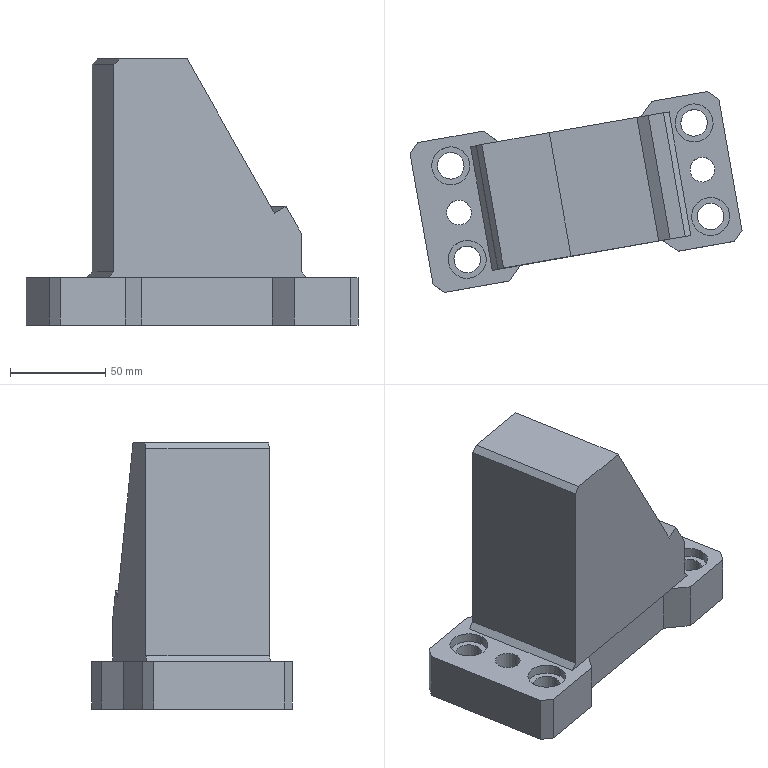Part | NX | features solid 2 | 1 solid | 46 faces | box 174.649 x 105.7 x 140 mm | volume 820537 mm3 | plane 36 | cylinder 10 | commonest cylinder face diameters 14 x4 20 x4 13 x2
STEP:
#1=CARTESIAN_POINT('',(-1147.121,323.745,25.));
#2=VERTEX_POINT('',#1);
#3=CARTESIAN_POINT('',(-1159.277,392.681,25.));
#4=VERTEX_POINT('',#3);
#5=CARTESIAN_POINT('',(-1153.199,358.213,25.));
#6=DIRECTION('',(-0.1736,0.9848,0.));
#7=VECTOR('',#6,1000.);
#8=LINE('',#5,#7);
#9=EDGE_CURVE('',#2,#4,#8,.T.);
#10=ORIENTED_EDGE('',*,*,#9,.F.);
#11=CARTESIAN_POINT('',(-1141.329,319.689,25.));
#12=VERTEX_POINT('',#11);
#13=CARTESIAN_POINT('',(-1119.608,304.48,25.));
#14=DIRECTION('',(-0.8192,0.5736,0.));
#15=VECTOR('',#14,1000.);
#16=LINE('',#13,#15);
#17=EDGE_CURVE('',#2,#12,#16,.F.);
#18=ORIENTED_EDGE('',*,*,#17,.T.);
#19=CARTESIAN_POINT('',(-1106.861,325.767,25.));
#20=VERTEX_POINT('',#19);
#21=CARTESIAN_POINT('',(-1065.007,333.147,25.));
#22=DIRECTION('',(-0.9848,-0.1736,0.));
#23=VECTOR('',#22,1000.);
#24=LINE('',#21,#23);
#25=EDGE_CURVE('',#20,#12,#24,.T.);
#26=ORIENTED_EDGE('',*,*,#25,.F.);
#27=CARTESIAN_POINT('',(-1101.183,333.876,25.));
#28=VERTEX_POINT('',#27);
#29=CARTESIAN_POINT('',(-1098.749,337.351,25.));
#30=DIRECTION('',(-0.5736,-0.8192,0.));
#31=VECTOR('',#30,1000.);
#32=LINE('',#29,#31);
#33=EDGE_CURVE('',#28,#20,#32,.T.);
#34=ORIENTED_EDGE('',*,*,#33,.F.);
#35=CARTESIAN_POINT('',(-1115.955,331.271,25.));
#36=VERTEX_POINT('',#35);
#37=CARTESIAN_POINT('',(-1113.,331.792,25.));
#38=DIRECTION('',(0.9848,0.1736,0.));
#39=VECTOR('',#38,1000.);
#40=LINE('',#37,#39);
#41=EDGE_CURVE('',#36,#28,#40,.T.);
#42=ORIENTED_EDGE('',*,*,#41,.F.);
#43=CARTESIAN_POINT('',(-1127.416,396.269,25.));
#44=VERTEX_POINT('',#43);
#45=CARTESIAN_POINT('',(-1127.416,396.269,25.));
#46=DIRECTION('',(-0.1736,0.9848,0.));
#47=VECTOR('',#46,1000.);
#48=LINE('',#45,#47);
#49=EDGE_CURVE('',#36,#44,#48,.T.);
#50=ORIENTED_EDGE('',*,*,#49,.T.);
#51=CARTESIAN_POINT('',(-1112.644,398.873,25.));
#52=VERTEX_POINT('',#51);
#53=CARTESIAN_POINT('',(-1124.461,396.79,25.));
#54=DIRECTION('',(0.9848,0.1736,0.));
#55=VECTOR('',#54,1000.);
#56=LINE('',#53,#55);
#57=EDGE_CURVE('',#44,#52,#56,.T.);
#58=ORIENTED_EDGE('',*,*,#57,.T.);
#59=CARTESIAN_POINT('',(-1120.753,404.551,25.));
#60=VERTEX_POINT('',#59);
#61=CARTESIAN_POINT('',(-1120.753,404.551,25.));
#62=DIRECTION('',(0.8192,-0.5736,0.));
#63=VECTOR('',#62,1000.);
#64=LINE('',#61,#63);
#65=EDGE_CURVE('',#60,#52,#64,.T.);
#66=ORIENTED_EDGE('',*,*,#65,.F.);
#67=CARTESIAN_POINT('',(-1155.221,398.474,25.));
#68=VERTEX_POINT('',#67);
#69=CARTESIAN_POINT('',(-1078.898,411.931,25.));
#70=DIRECTION('',(0.9848,0.1736,0.));
#71=VECTOR('',#70,1000.);
#72=LINE('',#69,#71);
#73=EDGE_CURVE('',#68,#60,#72,.T.);
#74=ORIENTED_EDGE('',*,*,#73,.F.);
#75=CARTESIAN_POINT('',(-1140.012,420.195,25.));
#76=DIRECTION('',(0.5736,0.8192,0.));
#77=VECTOR('',#76,1000.);
#78=LINE('',#75,#77);
#79=EDGE_CURVE('',#68,#4,#78,.F.);
#80=ORIENTED_EDGE('',*,*,#79,.T.);
#81=EDGE_LOOP('',(#10,#18,#26,#34,#42,#50,#58,#66,#74,#80));
#82=FACE_BOUND('',#81,.T.);
#83=CARTESIAN_POINT('',(-1127.996,388.043,25.));
#84=VERTEX_POINT('',#83);
#85=CARTESIAN_POINT('',(-1137.844,386.306,25.));
#86=DIRECTION('',(0.,0.,1.));
#87=DIRECTION('',(0.9848,0.1736,0.));
#88=AXIS2_PLACEMENT_3D('',#85,#86,#87);
#89=CIRCLE('',#88,10.);
#90=EDGE_CURVE('',#84,#84,#89,.T.);
#91=ORIENTED_EDGE('',*,*,#90,.F.);
#92=EDGE_LOOP('',(#91));
#93=FACE_BOUND('',#92,.T.);
#94=CARTESIAN_POINT('',(-1127.102,362.815,25.));
#95=VERTEX_POINT('',#94);
#96=CARTESIAN_POINT('',(-1133.503,361.686,25.));
#97=DIRECTION('',(0.,0.,1.));
#98=DIRECTION('',(0.9848,0.1736,0.));
#99=AXIS2_PLACEMENT_3D('',#96,#97,#98);
#100=CIRCLE('',#99,6.5);
#101=EDGE_CURVE('',#95,#95,#100,.T.);
#102=ORIENTED_EDGE('',*,*,#101,.F.);
#103=EDGE_LOOP('',(#102));
#104=FACE_BOUND('',#103,.T.);
#105=CARTESIAN_POINT('',(-1119.314,338.802,25.));
#106=VERTEX_POINT('',#105);
#107=CARTESIAN_POINT('',(-1129.162,337.066,25.));
#108=DIRECTION('',(0.,0.,1.));
#109=DIRECTION('',(0.9848,0.1736,0.));
#110=AXIS2_PLACEMENT_3D('',#107,#108,#109);
#111=CIRCLE('',#110,10.);
#112=EDGE_CURVE('',#106,#106,#111,.T.);
#113=ORIENTED_EDGE('',*,*,#112,.F.);
#114=EDGE_LOOP('',(#113));
#115=FACE_BOUND('',#114,.T.);
#116=CARTESIAN_POINT('',(-1071.952,372.539,25.));
#117=DIRECTION('',(0.,0.,1.));
#118=DIRECTION('',(0.9848,0.1736,0.));
#119=AXIS2_PLACEMENT_3D('',#116,#117,#118);
#120=PLANE('',#119);
#121=ADVANCED_FACE('',(#82,#93,#104,#115),#120,.T.);
#122=CARTESIAN_POINT('',(-996.784,421.333,25.));
#123=VERTEX_POINT('',#122);
#124=CARTESIAN_POINT('',(-984.628,352.397,25.));
#125=VERTEX_POINT('',#124);
#126=CARTESIAN_POINT('',(-990.706,386.865,25.));
#127=DIRECTION('',(0.1736,-0.9848,0.));
#128=VECTOR('',#127,1000.);
#129=LINE('',#126,#128);
#130=EDGE_CURVE('',#123,#125,#129,.T.);
#131=ORIENTED_EDGE('',*,*,#130,.F.);
#132=CARTESIAN_POINT('',(-1002.576,425.389,25.));
#133=VERTEX_POINT('',#132);
#134=CARTESIAN_POINT('',(-1024.297,440.598,25.));
#135=DIRECTION('',(0.8192,-0.5736,0.));
#136=VECTOR('',#135,1000.);
#137=LINE('',#134,#136);
#138=EDGE_CURVE('',#123,#133,#137,.F.);
#139=ORIENTED_EDGE('',*,*,#138,.T.);
#140=CARTESIAN_POINT('',(-1032.12,420.18,25.));
#141=VERTEX_POINT('',#140);
#142=CARTESIAN_POINT('',(-1078.898,411.931,25.));
#143=DIRECTION('',(0.9848,0.1736,0.));
#144=VECTOR('',#143,1000.);
#145=LINE('',#142,#144);
#146=EDGE_CURVE('',#141,#133,#145,.T.);
#147=ORIENTED_EDGE('',*,*,#146,.F.);
#148=CARTESIAN_POINT('',(-1037.798,412.071,25.));
#149=VERTEX_POINT('',#148);
#150=CARTESIAN_POINT('',(-1032.12,420.18,25.));
#151=DIRECTION('',(-0.5736,-0.8192,0.));
#152=VECTOR('',#151,1000.);
#153=LINE('',#150,#152);
#154=EDGE_CURVE('',#141,#149,#153,.T.);
#155=ORIENTED_EDGE('',*,*,#154,.T.);
#156=CARTESIAN_POINT('',(-1023.026,414.675,25.));
#157=VERTEX_POINT('',#156);
#158=CARTESIAN_POINT('',(-1124.461,396.79,25.));
#159=DIRECTION('',(0.9848,0.1736,0.));
#160=VECTOR('',#159,1000.);
#161=LINE('',#158,#160);
#162=EDGE_CURVE('',#149,#157,#161,.T.);
#163=ORIENTED_EDGE('',*,*,#162,.T.);
#164=CARTESIAN_POINT('',(-1011.565,349.678,25.));
#165=VERTEX_POINT('',#164);
#166=CARTESIAN_POINT('',(-1011.565,349.678,25.));
#167=DIRECTION('',(0.1736,-0.9848,0.));
#168=VECTOR('',#167,1000.);
#169=LINE('',#166,#168);
#170=EDGE_CURVE('',#157,#165,#169,.T.);
#171=ORIENTED_EDGE('',*,*,#170,.T.);
#172=CARTESIAN_POINT('',(-1026.337,347.073,25.));
#173=VERTEX_POINT('',#172);
#174=CARTESIAN_POINT('',(-1113.,331.792,25.));
#175=DIRECTION('',(0.9848,0.1736,0.));
#176=VECTOR('',#175,1000.);
#177=LINE('',#174,#176);
#178=EDGE_CURVE('',#173,#165,#177,.T.);
#179=ORIENTED_EDGE('',*,*,#178,.F.);
#180=CARTESIAN_POINT('',(-1018.228,341.395,25.));
#181=VERTEX_POINT('',#180);
#182=CARTESIAN_POINT('',(-1029.813,349.507,25.));
#183=DIRECTION('',(0.8192,-0.5736,0.));
#184=VECTOR('',#183,1000.);
#185=LINE('',#182,#184);
#186=EDGE_CURVE('',#173,#181,#185,.T.);
#187=ORIENTED_EDGE('',*,*,#186,.T.);
#188=CARTESIAN_POINT('',(-988.684,346.605,25.));
#189=VERTEX_POINT('',#188);
#190=CARTESIAN_POINT('',(-1065.007,333.147,25.));
#191=DIRECTION('',(-0.9848,-0.1736,0.));
#192=VECTOR('',#191,1000.);
#193=LINE('',#190,#192);
#194=EDGE_CURVE('',#189,#181,#193,.T.);
#195=ORIENTED_EDGE('',*,*,#194,.F.);
#196=CARTESIAN_POINT('',(-1003.893,324.884,25.));
#197=DIRECTION('',(-0.5736,-0.8192,0.));
#198=VECTOR('',#197,1000.);
#199=LINE('',#196,#198);
#200=EDGE_CURVE('',#189,#125,#199,.F.);
#201=ORIENTED_EDGE('',*,*,#200,.T.);
#202=EDGE_LOOP('',(#131,#139,#147,#155,#163,#171,#179,#187,#195,#201));
#203=FACE_BOUND('',#202,.T.);
#204=CARTESIAN_POINT('',(-999.971,410.617,25.));
#205=VERTEX_POINT('',#204);
#206=CARTESIAN_POINT('',(-1009.819,408.881,25.));
#207=DIRECTION('',(0.,0.,1.));
#208=DIRECTION('',(0.9848,0.1736,0.));
#209=AXIS2_PLACEMENT_3D('',#206,#207,#208);
#210=CIRCLE('',#209,10.);
#211=EDGE_CURVE('',#205,#205,#210,.T.);
#212=ORIENTED_EDGE('',*,*,#211,.F.);
#213=EDGE_LOOP('',(#212));
#214=FACE_BOUND('',#213,.T.);
#215=CARTESIAN_POINT('',(-999.077,385.389,25.));
#216=VERTEX_POINT('',#215);
#217=CARTESIAN_POINT('',(-1005.478,384.26,25.));
#218=DIRECTION('',(0.,0.,1.));
#219=DIRECTION('',(0.9848,0.1736,0.));
#220=AXIS2_PLACEMENT_3D('',#217,#218,#219);
#221=CIRCLE('',#220,6.5);
#222=EDGE_CURVE('',#216,#216,#221,.T.);
#223=ORIENTED_EDGE('',*,*,#222,.F.);
#224=EDGE_LOOP('',(#223));
#225=FACE_BOUND('',#224,.T.);
#226=CARTESIAN_POINT('',(-991.289,361.377,25.));
#227=VERTEX_POINT('',#226);
#228=CARTESIAN_POINT('',(-1001.137,359.64,25.));
#229=DIRECTION('',(0.,0.,1.));
#230=DIRECTION('',(0.9848,0.1736,0.));
#231=AXIS2_PLACEMENT_3D('',#228,#229,#230);
#232=CIRCLE('',#231,10.);
#233=EDGE_CURVE('',#227,#227,#232,.T.);
#234=ORIENTED_EDGE('',*,*,#233,.F.);
#235=EDGE_LOOP('',(#234));
#236=FACE_BOUND('',#235,.T.);
#237=CARTESIAN_POINT('',(-1071.952,372.539,25.));
#238=DIRECTION('',(0.,0.,1.));
#239=DIRECTION('',(0.9848,0.1736,0.));
#240=AXIS2_PLACEMENT_3D('',#237,#238,#239);
#241=PLANE('',#240);
#242=ADVANCED_FACE('',(#203,#214,#225,#236),#241,.T.);
#243=CARTESIAN_POINT('',(-1130.95,387.522,0.));
#244=VERTEX_POINT('',#243);
#245=CARTESIAN_POINT('',(-1137.844,386.306,0.));
#246=DIRECTION('',(0.,0.,1.));
#247=DIRECTION('',(0.9848,0.1736,0.));
#248=AXIS2_PLACEMENT_3D('',#245,#246,#247);
#249=CIRCLE('',#248,7.);
#250=EDGE_CURVE('',#244,#244,#249,.T.);
#251=ORIENTED_EDGE('',*,*,#250,.F.);
#252=EDGE_LOOP('',(#251));
#253=FACE_BOUND('',#252,.T.);
#254=CARTESIAN_POINT('',(-1144.738,385.091,20.));
#255=VERTEX_POINT('',#254);
#256=CARTESIAN_POINT('',(-1137.844,386.306,20.));
#257=DIRECTION('',(0.,0.,1.));
#258=DIRECTION('',(-0.9848,-0.1736,0.));
#259=AXIS2_PLACEMENT_3D('',#256,#257,#258);
#260=CIRCLE('',#259,7.);
#261=EDGE_CURVE('',#255,#255,#260,.T.);
#262=ORIENTED_EDGE('',*,*,#261,.T.);
#263=EDGE_LOOP('',(#262));
#264=FACE_BOUND('',#263,.T.);
#265=CARTESIAN_POINT('',(-1137.844,386.306,25.));
#266=DIRECTION('',(0.,0.,-1.));
#267=DIRECTION('',(-0.1736,0.9848,0.));
#268=AXIS2_PLACEMENT_3D('',#265,#266,#267);
#269=CYLINDRICAL_SURFACE('',#268,7.);
#270=ADVANCED_FACE('',(#253,#264),#269,.F.);
#271=CARTESIAN_POINT('',(-1122.268,338.282,0.));
#272=VERTEX_POINT('',#271);
#273=CARTESIAN_POINT('',(-1129.162,337.066,0.));
#274=DIRECTION('',(0.,0.,1.));
#275=DIRECTION('',(0.9848,0.1736,0.));
#276=AXIS2_PLACEMENT_3D('',#273,#274,#275);
#277=CIRCLE('',#276,7.);
#278=EDGE_CURVE('',#272,#272,#277,.T.);
#279=ORIENTED_EDGE('',*,*,#278,.F.);
#280=EDGE_LOOP('',(#279));
#281=FACE_BOUND('',#280,.T.);
#282=CARTESIAN_POINT('',(-1136.055,335.85,20.));
#283=VERTEX_POINT('',#282);
#284=CARTESIAN_POINT('',(-1129.162,337.066,20.));
#285=DIRECTION('',(0.,0.,1.));
#286=DIRECTION('',(-0.9848,-0.1736,0.));
#287=AXIS2_PLACEMENT_3D('',#284,#285,#286);
#288=CIRCLE('',#287,7.);
#289=EDGE_CURVE('',#283,#283,#288,.T.);
#290=ORIENTED_EDGE('',*,*,#289,.T.);
#291=EDGE_LOOP('',(#290));
#292=FACE_BOUND('',#291,.T.);
#293=CARTESIAN_POINT('',(-1129.162,337.066,25.));
#294=DIRECTION('',(0.,0.,-1.));
#295=DIRECTION('',(-0.1736,0.9848,0.));
#296=AXIS2_PLACEMENT_3D('',#293,#294,#295);
#297=CYLINDRICAL_SURFACE('',#296,7.);
#298=ADVANCED_FACE('',(#281,#292),#297,.F.);
#299=CARTESIAN_POINT('',(-994.243,360.856,0.));
#300=VERTEX_POINT('',#299);
#301=CARTESIAN_POINT('',(-1001.137,359.64,0.));
#302=DIRECTION('',(0.,0.,1.));
#303=DIRECTION('',(0.9848,0.1736,0.));
#304=AXIS2_PLACEMENT_3D('',#301,#302,#303);
#305=CIRCLE('',#304,7.);
#306=EDGE_CURVE('',#300,#300,#305,.T.);
#307=ORIENTED_EDGE('',*,*,#306,.F.);
#308=EDGE_LOOP('',(#307));
#309=FACE_BOUND('',#308,.T.);
#310=CARTESIAN_POINT('',(-1008.03,358.425,20.));
#311=VERTEX_POINT('',#310);
#312=CARTESIAN_POINT('',(-1001.137,359.64,20.));
#313=DIRECTION('',(0.,0.,1.));
#314=DIRECTION('',(-0.9848,-0.1736,0.));
#315=AXIS2_PLACEMENT_3D('',#312,#313,#314);
#316=CIRCLE('',#315,7.);
#317=EDGE_CURVE('',#311,#311,#316,.T.);
#318=ORIENTED_EDGE('',*,*,#317,.T.);
#319=EDGE_LOOP('',(#318));
#320=FACE_BOUND('',#319,.T.);
#321=CARTESIAN_POINT('',(-1001.137,359.64,25.));
#322=DIRECTION('',(0.,0.,-1.));
#323=DIRECTION('',(-0.1736,0.9848,0.));
#324=AXIS2_PLACEMENT_3D('',#321,#322,#323);
#325=CYLINDRICAL_SURFACE('',#324,7.);
#326=ADVANCED_FACE('',(#309,#320),#325,.F.);
#327=CARTESIAN_POINT('',(-1002.925,410.096,0.));
#328=VERTEX_POINT('',#327);
#329=CARTESIAN_POINT('',(-1009.819,408.881,0.));
#330=DIRECTION('',(0.,0.,1.));
#331=DIRECTION('',(0.9848,0.1736,0.));
#332=AXIS2_PLACEMENT_3D('',#329,#330,#331);
#333=CIRCLE('',#332,7.);
#334=EDGE_CURVE('',#328,#328,#333,.T.);
#335=ORIENTED_EDGE('',*,*,#334,.F.);
#336=EDGE_LOOP('',(#335));
#337=FACE_BOUND('',#336,.T.);
#338=CARTESIAN_POINT('',(-1016.713,407.665,20.));
#339=VERTEX_POINT('',#338);
#340=CARTESIAN_POINT('',(-1009.819,408.881,20.));
#341=DIRECTION('',(0.,0.,1.));
#342=DIRECTION('',(-0.9848,-0.1736,0.));
#343=AXIS2_PLACEMENT_3D('',#340,#341,#342);
#344=CIRCLE('',#343,7.);
#345=EDGE_CURVE('',#339,#339,#344,.T.);
#346=ORIENTED_EDGE('',*,*,#345,.T.);
#347=EDGE_LOOP('',(#346));
#348=FACE_BOUND('',#347,.T.);
#349=CARTESIAN_POINT('',(-1009.819,408.881,25.));
#350=DIRECTION('',(0.,0.,-1.));
#351=DIRECTION('',(-0.1736,0.9848,0.));
#352=AXIS2_PLACEMENT_3D('',#349,#350,#351);
#353=CYLINDRICAL_SURFACE('',#352,7.);
#354=ADVANCED_FACE('',(#337,#348),#353,.F.);
#355=CARTESIAN_POINT('',(-1127.102,362.815,0.));
#356=VERTEX_POINT('',#355);
#357=CARTESIAN_POINT('',(-1133.503,361.686,0.));
#358=DIRECTION('',(0.,0.,1.));
#359=DIRECTION('',(0.9848,0.1736,0.));
#360=AXIS2_PLACEMENT_3D('',#357,#358,#359);
#361=CIRCLE('',#360,6.5);
#362=EDGE_CURVE('',#356,#356,#361,.T.);
#363=ORIENTED_EDGE('',*,*,#362,.T.);
#364=EDGE_LOOP('',(#363));
#365=FACE_BOUND('',#364,.T.);
#366=ORIENTED_EDGE('',*,*,#306,.T.);
#367=EDGE_LOOP('',(#366));
#368=FACE_BOUND('',#367,.T.);
#369=ORIENTED_EDGE('',*,*,#334,.T.);
#370=EDGE_LOOP('',(#369));
#371=FACE_BOUND('',#370,.T.);
#372=CARTESIAN_POINT('',(-1002.576,425.389,0.));
#373=VERTEX_POINT('',#372);
#374=CARTESIAN_POINT('',(-1032.12,420.18,0.));
#375=VERTEX_POINT('',#374);
#376=CARTESIAN_POINT('',(-1078.898,411.931,0.));
#377=DIRECTION('',(-0.9848,-0.1736,0.));
#378=VECTOR('',#377,1000.);
#379=LINE('',#376,#378);
#380=EDGE_CURVE('',#373,#375,#379,.T.);
#381=ORIENTED_EDGE('',*,*,#380,.F.);
#382=CARTESIAN_POINT('',(-996.784,421.333,0.));
#383=VERTEX_POINT('',#382);
#384=CARTESIAN_POINT('',(-1024.297,440.598,0.));
#385=DIRECTION('',(-0.8192,0.5736,0.));
#386=VECTOR('',#385,1000.);
#387=LINE('',#384,#386);
#388=EDGE_CURVE('',#373,#383,#387,.F.);
#389=ORIENTED_EDGE('',*,*,#388,.T.);
#390=CARTESIAN_POINT('',(-984.628,352.397,0.));
#391=VERTEX_POINT('',#390);
#392=CARTESIAN_POINT('',(-990.706,386.865,0.));
#393=DIRECTION('',(-0.1736,0.9848,0.));
#394=VECTOR('',#393,1000.);
#395=LINE('',#392,#394);
#396=EDGE_CURVE('',#391,#383,#395,.T.);
#397=ORIENTED_EDGE('',*,*,#396,.F.);
#398=CARTESIAN_POINT('',(-988.684,346.605,0.));
#399=VERTEX_POINT('',#398);
#400=CARTESIAN_POINT('',(-1003.893,324.884,0.));
#401=DIRECTION('',(0.5736,0.8192,0.));
#402=VECTOR('',#401,1000.);
#403=LINE('',#400,#402);
#404=EDGE_CURVE('',#391,#399,#403,.F.);
#405=ORIENTED_EDGE('',*,*,#404,.T.);
#406=CARTESIAN_POINT('',(-1018.228,341.395,0.));
#407=VERTEX_POINT('',#406);
#408=CARTESIAN_POINT('',(-1065.007,333.147,0.));
#409=DIRECTION('',(0.9848,0.1736,0.));
#410=VECTOR('',#409,1000.);
#411=LINE('',#408,#410);
#412=EDGE_CURVE('',#407,#399,#411,.T.);
#413=ORIENTED_EDGE('',*,*,#412,.F.);
#414=CARTESIAN_POINT('',(-1029.813,349.507,0.));
#415=VERTEX_POINT('',#414);
#416=CARTESIAN_POINT('',(-1029.813,349.507,0.));
#417=DIRECTION('',(0.8192,-0.5736,0.));
#418=VECTOR('',#417,1000.);
#419=LINE('',#416,#418);
#420=EDGE_CURVE('',#415,#407,#419,.T.);
#421=ORIENTED_EDGE('',*,*,#420,.F.);
#422=CARTESIAN_POINT('',(-1098.749,337.351,0.));
#423=VERTEX_POINT('',#422);
#424=CARTESIAN_POINT('',(-1098.749,337.351,0.));
#425=DIRECTION('',(0.9848,0.1736,0.));
#426=VECTOR('',#425,1000.);
#427=LINE('',#424,#426);
#428=EDGE_CURVE('',#423,#415,#427,.T.);
#429=ORIENTED_EDGE('',*,*,#428,.F.);
#430=CARTESIAN_POINT('',(-1106.861,325.767,0.));
#431=VERTEX_POINT('',#430);
#432=CARTESIAN_POINT('',(-1098.749,337.351,0.));
#433=DIRECTION('',(-0.5736,-0.8192,0.));
#434=VECTOR('',#433,1000.);
#435=LINE('',#432,#434);
#436=EDGE_CURVE('',#423,#431,#435,.T.);
#437=ORIENTED_EDGE('',*,*,#436,.T.);
#438=CARTESIAN_POINT('',(-1141.329,319.689,0.));
#439=VERTEX_POINT('',#438);
#440=CARTESIAN_POINT('',(-1065.007,333.147,0.));
#441=DIRECTION('',(0.9848,0.1736,0.));
#442=VECTOR('',#441,1000.);
#443=LINE('',#440,#442);
#444=EDGE_CURVE('',#439,#431,#443,.T.);
#445=ORIENTED_EDGE('',*,*,#444,.F.);
#446=CARTESIAN_POINT('',(-1147.121,323.745,0.));
#447=VERTEX_POINT('',#446);
#448=CARTESIAN_POINT('',(-1119.608,304.48,0.));
#449=DIRECTION('',(0.8192,-0.5736,0.));
#450=VECTOR('',#449,1000.);
#451=LINE('',#448,#450);
#452=EDGE_CURVE('',#439,#447,#451,.F.);
#453=ORIENTED_EDGE('',*,*,#452,.T.);
#454=CARTESIAN_POINT('',(-1159.277,392.681,0.));
#455=VERTEX_POINT('',#454);
#456=CARTESIAN_POINT('',(-1153.199,358.213,0.));
#457=DIRECTION('',(0.1736,-0.9848,0.));
#458=VECTOR('',#457,1000.);
#459=LINE('',#456,#458);
#460=EDGE_CURVE('',#455,#447,#459,.T.);
#461=ORIENTED_EDGE('',*,*,#460,.F.);
#462=CARTESIAN_POINT('',(-1155.221,398.474,0.));
#463=VERTEX_POINT('',#462);
#464=CARTESIAN_POINT('',(-1140.012,420.195,0.));
#465=DIRECTION('',(-0.5736,-0.8192,0.));
#466=VECTOR('',#465,1000.);
#467=LINE('',#464,#466);
#468=EDGE_CURVE('',#455,#463,#467,.F.);
#469=ORIENTED_EDGE('',*,*,#468,.T.);
#470=CARTESIAN_POINT('',(-1120.753,404.551,0.));
#471=VERTEX_POINT('',#470);
#472=CARTESIAN_POINT('',(-1078.898,411.931,0.));
#473=DIRECTION('',(-0.9848,-0.1736,0.));
#474=VECTOR('',#473,1000.);
#475=LINE('',#472,#474);
#476=EDGE_CURVE('',#471,#463,#475,.T.);
#477=ORIENTED_EDGE('',*,*,#476,.F.);
#478=CARTESIAN_POINT('',(-1109.168,396.44,0.));
#479=VERTEX_POINT('',#478);
#480=CARTESIAN_POINT('',(-1120.753,404.551,0.));
#481=DIRECTION('',(0.8192,-0.5736,0.));
#482=VECTOR('',#481,1000.);
#483=LINE('',#480,#482);
#484=EDGE_CURVE('',#471,#479,#483,.T.);
#485=ORIENTED_EDGE('',*,*,#484,.T.);
#486=CARTESIAN_POINT('',(-1040.232,408.595,0.));
#487=VERTEX_POINT('',#486);
#488=CARTESIAN_POINT('',(-1109.168,396.44,0.));
#489=DIRECTION('',(0.9848,0.1736,0.));
#490=VECTOR('',#489,1000.);
#491=LINE('',#488,#490);
#492=EDGE_CURVE('',#479,#487,#491,.T.);
#493=ORIENTED_EDGE('',*,*,#492,.T.);
#494=CARTESIAN_POINT('',(-1032.12,420.18,0.));
#495=DIRECTION('',(-0.5736,-0.8192,0.));
#496=VECTOR('',#495,1000.);
#497=LINE('',#494,#496);
#498=EDGE_CURVE('',#375,#487,#497,.T.);
#499=ORIENTED_EDGE('',*,*,#498,.F.);
#500=EDGE_LOOP('',(#381,#389,#397,#405,#413,#421,#429,#437,#445,#453,#461,#469,#477,#485,#493,#499));
#501=FACE_BOUND('',#500,.T.);
#502=CARTESIAN_POINT('',(-999.077,385.389,0.));
#503=VERTEX_POINT('',#502);
#504=CARTESIAN_POINT('',(-1005.478,384.26,0.));
#505=DIRECTION('',(0.,0.,1.));
#506=DIRECTION('',(0.9848,0.1736,0.));
#507=AXIS2_PLACEMENT_3D('',#504,#505,#506);
#508=CIRCLE('',#507,6.5);
#509=EDGE_CURVE('',#503,#503,#508,.T.);
#510=ORIENTED_EDGE('',*,*,#509,.T.);
#511=EDGE_LOOP('',(#510));
#512=FACE_BOUND('',#511,.T.);
#513=ORIENTED_EDGE('',*,*,#250,.T.);
#514=EDGE_LOOP('',(#513));
#515=FACE_BOUND('',#514,.T.);
#516=ORIENTED_EDGE('',*,*,#278,.T.);
#517=EDGE_LOOP('',(#516));
#518=FACE_BOUND('',#517,.T.);
#519=CARTESIAN_POINT('',(-1071.952,372.539,0.));
#520=DIRECTION('',(0.,0.,-1.));
#521=DIRECTION('',(-0.9848,-0.1736,0.));
#522=AXIS2_PLACEMENT_3D('',#519,#520,#521);
#523=PLANE('',#522);
#524=ADVANCED_FACE('',(#365,#368,#371,#501,#512,#515,#518),#523,.T.);
#525=ORIENTED_EDGE('',*,*,#25,.T.);
#526=CARTESIAN_POINT('',(-1141.329,319.689,0.));
#527=DIRECTION('',(0.,0.,-1.));
#528=VECTOR('',#527,1000.);
#529=LINE('',#526,#528);
#530=EDGE_CURVE('',#12,#439,#529,.T.);
#531=ORIENTED_EDGE('',*,*,#530,.T.);
#532=ORIENTED_EDGE('',*,*,#444,.T.);
#533=CARTESIAN_POINT('',(-1106.861,325.767,25.));
#534=DIRECTION('',(0.,0.,-1.));
#535=VECTOR('',#534,1000.);
#536=LINE('',#533,#535);
#537=EDGE_CURVE('',#20,#431,#536,.T.);
#538=ORIENTED_EDGE('',*,*,#537,.F.);
#539=EDGE_LOOP('',(#525,#531,#532,#538));
#540=FACE_BOUND('',#539,.T.);
#541=CARTESIAN_POINT('',(-1065.007,333.147,0.));
#542=DIRECTION('',(0.1736,-0.9848,0.));
#543=DIRECTION('',(0.,0.,-1.));
#544=AXIS2_PLACEMENT_3D('',#541,#542,#543);
#545=PLANE('',#544);
#546=ADVANCED_FACE('',(#540),#545,.T.);
#547=ORIENTED_EDGE('',*,*,#476,.T.);
#548=CARTESIAN_POINT('',(-1155.221,398.474,0.));
#549=DIRECTION('',(0.,0.,1.));
#550=VECTOR('',#549,1000.);
#551=LINE('',#548,#550);
#552=EDGE_CURVE('',#463,#68,#551,.T.);
#553=ORIENTED_EDGE('',*,*,#552,.T.);
#554=ORIENTED_EDGE('',*,*,#73,.T.);
#555=CARTESIAN_POINT('',(-1120.753,404.551,25.));
#556=DIRECTION('',(0.,0.,-1.));
#557=VECTOR('',#556,1000.);
#558=LINE('',#555,#557);
#559=EDGE_CURVE('',#60,#471,#558,.T.);
#560=ORIENTED_EDGE('',*,*,#559,.T.);
#561=EDGE_LOOP('',(#547,#553,#554,#560));
#562=FACE_BOUND('',#561,.T.);
#563=CARTESIAN_POINT('',(-1078.898,411.931,0.));
#564=DIRECTION('',(-0.1736,0.9848,0.));
#565=DIRECTION('',(0.,0.,1.));
#566=AXIS2_PLACEMENT_3D('',#563,#564,#565);
#567=PLANE('',#566);
#568=ADVANCED_FACE('',(#562),#567,.T.);
#569=ORIENTED_EDGE('',*,*,#412,.T.);
#570=CARTESIAN_POINT('',(-988.684,346.605,0.));
#571=DIRECTION('',(0.,0.,1.));
#572=VECTOR('',#571,1000.);
#573=LINE('',#570,#572);
#574=EDGE_CURVE('',#399,#189,#573,.T.);
#575=ORIENTED_EDGE('',*,*,#574,.T.);
#576=ORIENTED_EDGE('',*,*,#194,.T.);
#577=CARTESIAN_POINT('',(-1018.228,341.395,25.));
#578=DIRECTION('',(0.,0.,-1.));
#579=VECTOR('',#578,1000.);
#580=LINE('',#577,#579);
#581=EDGE_CURVE('',#181,#407,#580,.T.);
#582=ORIENTED_EDGE('',*,*,#581,.T.);
#583=EDGE_LOOP('',(#569,#575,#576,#582));
#584=FACE_BOUND('',#583,.T.);
#585=CARTESIAN_POINT('',(-1065.007,333.147,0.));
#586=DIRECTION('',(0.1736,-0.9848,0.));
#587=DIRECTION('',(0.,0.,-1.));
#588=AXIS2_PLACEMENT_3D('',#585,#586,#587);
#589=PLANE('',#588);
#590=ADVANCED_FACE('',(#584),#589,.T.);
#591=ORIENTED_EDGE('',*,*,#460,.T.);
#592=CARTESIAN_POINT('',(-1147.121,323.745,0.));
#593=DIRECTION('',(0.,0.,1.));
#594=VECTOR('',#593,1000.);
#595=LINE('',#592,#594);
#596=EDGE_CURVE('',#447,#2,#595,.T.);
#597=ORIENTED_EDGE('',*,*,#596,.T.);
#598=ORIENTED_EDGE('',*,*,#9,.T.);
#599=CARTESIAN_POINT('',(-1159.277,392.681,0.));
#600=DIRECTION('',(0.,0.,-1.));
#601=VECTOR('',#600,1000.);
#602=LINE('',#599,#601);
#603=EDGE_CURVE('',#4,#455,#602,.T.);
#604=ORIENTED_EDGE('',*,*,#603,.T.);
#605=EDGE_LOOP('',(#591,#597,#598,#604));
#606=FACE_BOUND('',#605,.T.);
#607=CARTESIAN_POINT('',(-1153.199,358.213,0.));
#608=DIRECTION('',(-0.9848,-0.1736,0.));
#609=DIRECTION('',(0.,0.,1.));
#610=AXIS2_PLACEMENT_3D('',#607,#608,#609);
#611=PLANE('',#610);
#612=ADVANCED_FACE('',(#606),#611,.T.);
#613=ORIENTED_EDGE('',*,*,#146,.T.);
#614=CARTESIAN_POINT('',(-1002.576,425.389,0.));
#615=DIRECTION('',(0.,0.,-1.));
#616=VECTOR('',#615,1000.);
#617=LINE('',#614,#616);
#618=EDGE_CURVE('',#133,#373,#617,.T.);
#619=ORIENTED_EDGE('',*,*,#618,.T.);
#620=ORIENTED_EDGE('',*,*,#380,.T.);
#621=CARTESIAN_POINT('',(-1032.12,420.18,25.));
#622=DIRECTION('',(0.,0.,-1.));
#623=VECTOR('',#622,1000.);
#624=LINE('',#621,#623);
#625=EDGE_CURVE('',#141,#375,#624,.T.);
#626=ORIENTED_EDGE('',*,*,#625,.F.);
#627=EDGE_LOOP('',(#613,#619,#620,#626));
#628=FACE_BOUND('',#627,.T.);
#629=CARTESIAN_POINT('',(-1078.898,411.931,0.));
#630=DIRECTION('',(-0.1736,0.9848,0.));
#631=DIRECTION('',(0.,0.,1.));
#632=AXIS2_PLACEMENT_3D('',#629,#630,#631);
#633=PLANE('',#632);
#634=ADVANCED_FACE('',(#628),#633,.T.);
#635=ORIENTED_EDGE('',*,*,#396,.T.);
#636=CARTESIAN_POINT('',(-996.784,421.333,0.));
#637=DIRECTION('',(0.,0.,1.));
#638=VECTOR('',#637,1000.);
#639=LINE('',#636,#638);
#640=EDGE_CURVE('',#383,#123,#639,.T.);
#641=ORIENTED_EDGE('',*,*,#640,.T.);
#642=ORIENTED_EDGE('',*,*,#130,.T.);
#643=CARTESIAN_POINT('',(-984.628,352.397,0.));
#644=DIRECTION('',(0.,0.,-1.));
#645=VECTOR('',#644,1000.);
#646=LINE('',#643,#645);
#647=EDGE_CURVE('',#125,#391,#646,.T.);
#648=ORIENTED_EDGE('',*,*,#647,.T.);
#649=EDGE_LOOP('',(#635,#641,#642,#648));
#650=FACE_BOUND('',#649,.T.);
#651=CARTESIAN_POINT('',(-990.706,386.865,0.));
#652=DIRECTION('',(0.9848,0.1736,0.));
#653=DIRECTION('',(0.,0.,-1.));
#654=AXIS2_PLACEMENT_3D('',#651,#652,#653);
#655=PLANE('',#654);
#656=ADVANCED_FACE('',(#650),#655,.T.);
#657=ORIENTED_EDGE('',*,*,#498,.T.);
#658=CARTESIAN_POINT('',(-1040.232,408.595,25.));
#659=VERTEX_POINT('',#658);
#660=CARTESIAN_POINT('',(-1040.232,408.595,25.));
#661=DIRECTION('',(0.,0.,-1.));
#662=VECTOR('',#661,1000.);
#663=LINE('',#660,#662);
#664=EDGE_CURVE('',#659,#487,#663,.T.);
#665=ORIENTED_EDGE('',*,*,#664,.F.);
#666=CARTESIAN_POINT('',(-1032.12,420.18,25.));
#667=DIRECTION('',(-0.5736,-0.8192,0.));
#668=VECTOR('',#667,1000.);
#669=LINE('',#666,#668);
#670=EDGE_CURVE('',#149,#659,#669,.T.);
#671=ORIENTED_EDGE('',*,*,#670,.F.);
#672=ORIENTED_EDGE('',*,*,#154,.F.);
#673=ORIENTED_EDGE('',*,*,#625,.T.);
#674=EDGE_LOOP('',(#657,#665,#671,#672,#673));
#675=FACE_BOUND('',#674,.T.);
#676=CARTESIAN_POINT('',(-1032.12,420.18,25.));
#677=DIRECTION('',(0.8192,-0.5736,0.));
#678=DIRECTION('',(0.5736,0.8192,0.));
#679=AXIS2_PLACEMENT_3D('',#676,#677,#678);
#680=PLANE('',#679);
#681=ADVANCED_FACE('',(#675),#680,.F.);
#682=ORIENTED_EDGE('',*,*,#492,.F.);
#683=CARTESIAN_POINT('',(-1109.168,396.44,25.));
#684=VERTEX_POINT('',#683);
#685=CARTESIAN_POINT('',(-1109.168,396.44,25.));
#686=DIRECTION('',(0.,0.,-1.));
#687=VECTOR('',#686,1000.);
#688=LINE('',#685,#687);
#689=EDGE_CURVE('',#684,#479,#688,.T.);
#690=ORIENTED_EDGE('',*,*,#689,.F.);
#691=CARTESIAN_POINT('',(-1109.168,396.44,25.));
#692=DIRECTION('',(0.9848,0.1736,0.));
#693=VECTOR('',#692,1000.);
#694=LINE('',#691,#693);
#695=EDGE_CURVE('',#684,#659,#694,.T.);
#696=ORIENTED_EDGE('',*,*,#695,.T.);
#697=ORIENTED_EDGE('',*,*,#664,.T.);
#698=EDGE_LOOP('',(#682,#690,#696,#697));
#699=FACE_BOUND('',#698,.T.);
#700=CARTESIAN_POINT('',(-1109.168,396.44,25.));
#701=DIRECTION('',(-0.1736,0.9848,0.));
#702=DIRECTION('',(-0.9848,-0.1736,0.));
#703=AXIS2_PLACEMENT_3D('',#700,#701,#702);
#704=PLANE('',#703);
#705=ADVANCED_FACE('',(#699),#704,.T.);
#706=ORIENTED_EDGE('',*,*,#484,.F.);
#707=ORIENTED_EDGE('',*,*,#559,.F.);
#708=ORIENTED_EDGE('',*,*,#65,.T.);
#709=CARTESIAN_POINT('',(-1120.753,404.551,25.));
#710=DIRECTION('',(0.8192,-0.5736,0.));
#711=VECTOR('',#710,1000.);
#712=LINE('',#709,#711);
#713=EDGE_CURVE('',#52,#684,#712,.T.);
#714=ORIENTED_EDGE('',*,*,#713,.T.);
#715=ORIENTED_EDGE('',*,*,#689,.T.);
#716=EDGE_LOOP('',(#706,#707,#708,#714,#715));
#717=FACE_BOUND('',#716,.T.);
#718=CARTESIAN_POINT('',(-1120.753,404.551,25.));
#719=DIRECTION('',(0.5736,0.8192,0.));
#720=DIRECTION('',(-0.8192,0.5736,0.));
#721=AXIS2_PLACEMENT_3D('',#718,#719,#720);
#722=PLANE('',#721);
#723=ADVANCED_FACE('',(#717),#722,.T.);
#724=ORIENTED_EDGE('',*,*,#420,.T.);
#725=ORIENTED_EDGE('',*,*,#581,.F.);
#726=ORIENTED_EDGE('',*,*,#186,.F.);
#727=CARTESIAN_POINT('',(-1029.813,349.507,25.));
#728=VERTEX_POINT('',#727);
#729=CARTESIAN_POINT('',(-1029.813,349.507,25.));
#730=DIRECTION('',(0.8192,-0.5736,0.));
#731=VECTOR('',#730,1000.);
#732=LINE('',#729,#731);
#733=EDGE_CURVE('',#728,#173,#732,.T.);
#734=ORIENTED_EDGE('',*,*,#733,.F.);
#735=CARTESIAN_POINT('',(-1029.813,349.507,25.));
#736=DIRECTION('',(0.,0.,-1.));
#737=VECTOR('',#736,1000.);
#738=LINE('',#735,#737);
#739=EDGE_CURVE('',#728,#415,#738,.T.);
#740=ORIENTED_EDGE('',*,*,#739,.T.);
#741=EDGE_LOOP('',(#724,#725,#726,#734,#740));
#742=FACE_BOUND('',#741,.T.);
#743=CARTESIAN_POINT('',(-1029.813,349.507,25.));
#744=DIRECTION('',(0.5736,0.8192,0.));
#745=DIRECTION('',(-0.8192,0.5736,0.));
#746=AXIS2_PLACEMENT_3D('',#743,#744,#745);
#747=PLANE('',#746);
#748=ADVANCED_FACE('',(#742),#747,.F.);
#749=ORIENTED_EDGE('',*,*,#436,.F.);
#750=CARTESIAN_POINT('',(-1098.749,337.351,25.));
#751=VERTEX_POINT('',#750);
#752=CARTESIAN_POINT('',(-1098.749,337.351,25.));
#753=DIRECTION('',(0.,0.,-1.));
#754=VECTOR('',#753,1000.);
#755=LINE('',#752,#754);
#756=EDGE_CURVE('',#751,#423,#755,.T.);
#757=ORIENTED_EDGE('',*,*,#756,.F.);
#758=CARTESIAN_POINT('',(-1098.749,337.351,25.));
#759=DIRECTION('',(-0.5736,-0.8192,0.));
#760=VECTOR('',#759,1000.);
#761=LINE('',#758,#760);
#762=EDGE_CURVE('',#751,#28,#761,.T.);
#763=ORIENTED_EDGE('',*,*,#762,.T.);
#764=ORIENTED_EDGE('',*,*,#33,.T.);
#765=ORIENTED_EDGE('',*,*,#537,.T.);
#766=EDGE_LOOP('',(#749,#757,#763,#764,#765));
#767=FACE_BOUND('',#766,.T.);
#768=CARTESIAN_POINT('',(-1098.749,337.351,25.));
#769=DIRECTION('',(0.8192,-0.5736,0.));
#770=DIRECTION('',(0.5736,0.8192,0.));
#771=AXIS2_PLACEMENT_3D('',#768,#769,#770);
#772=PLANE('',#771);
#773=ADVANCED_FACE('',(#767),#772,.T.);
#774=ORIENTED_EDGE('',*,*,#428,.T.);
#775=ORIENTED_EDGE('',*,*,#739,.F.);
#776=CARTESIAN_POINT('',(-1098.749,337.351,25.));
#777=DIRECTION('',(0.9848,0.1736,0.));
#778=VECTOR('',#777,1000.);
#779=LINE('',#776,#778);
#780=EDGE_CURVE('',#751,#728,#779,.T.);
#781=ORIENTED_EDGE('',*,*,#780,.F.);
#782=ORIENTED_EDGE('',*,*,#756,.T.);
#783=EDGE_LOOP('',(#774,#775,#781,#782));
#784=FACE_BOUND('',#783,.T.);
#785=CARTESIAN_POINT('',(-1098.749,337.351,25.));
#786=DIRECTION('',(-0.1736,0.9848,0.));
#787=DIRECTION('',(-0.9848,-0.1736,0.));
#788=AXIS2_PLACEMENT_3D('',#785,#786,#787);
#789=PLANE('',#788);
#790=ADVANCED_FACE('',(#784),#789,.F.);
#791=ORIENTED_EDGE('',*,*,#222,.T.);
#792=EDGE_LOOP('',(#791));
#793=FACE_BOUND('',#792,.T.);
#794=ORIENTED_EDGE('',*,*,#509,.F.);
#795=EDGE_LOOP('',(#794));
#796=FACE_BOUND('',#795,.T.);
#797=CARTESIAN_POINT('',(-1005.478,384.26,25.));
#798=DIRECTION('',(0.,0.,-1.));
#799=DIRECTION('',(-0.1736,0.9848,0.));
#800=AXIS2_PLACEMENT_3D('',#797,#798,#799);
#801=CYLINDRICAL_SURFACE('',#800,6.5);
#802=ADVANCED_FACE('',(#793,#796),#801,.F.);
#803=ORIENTED_EDGE('',*,*,#101,.T.);
#804=EDGE_LOOP('',(#803));
#805=FACE_BOUND('',#804,.T.);
#806=ORIENTED_EDGE('',*,*,#362,.F.);
#807=EDGE_LOOP('',(#806));
#808=FACE_BOUND('',#807,.T.);
#809=CARTESIAN_POINT('',(-1133.503,361.686,25.));
#810=DIRECTION('',(0.,0.,-1.));
#811=DIRECTION('',(-0.1736,0.9848,0.));
#812=AXIS2_PLACEMENT_3D('',#809,#810,#811);
#813=CYLINDRICAL_SURFACE('',#812,6.5);
#814=ADVANCED_FACE('',(#805,#808),#813,.F.);
#815=ORIENTED_EDGE('',*,*,#211,.T.);
#816=EDGE_LOOP('',(#815));
#817=FACE_BOUND('',#816,.T.);
#818=CARTESIAN_POINT('',(-999.971,410.617,20.));
#819=VERTEX_POINT('',#818);
#820=CARTESIAN_POINT('',(-1009.819,408.881,20.));
#821=DIRECTION('',(0.,0.,1.));
#822=DIRECTION('',(0.9848,0.1736,0.));
#823=AXIS2_PLACEMENT_3D('',#820,#821,#822);
#824=CIRCLE('',#823,10.);
#825=EDGE_CURVE('',#819,#819,#824,.T.);
#826=ORIENTED_EDGE('',*,*,#825,.F.);
#827=EDGE_LOOP('',(#826));
#828=FACE_BOUND('',#827,.T.);
#829=CARTESIAN_POINT('',(-1009.819,408.881,25.));
#830=DIRECTION('',(0.,0.,-1.));
#831=DIRECTION('',(-0.1736,0.9848,0.));
#832=AXIS2_PLACEMENT_3D('',#829,#830,#831);
#833=CYLINDRICAL_SURFACE('',#832,10.);
#834=ADVANCED_FACE('',(#817,#828),#833,.F.);
#835=ORIENTED_EDGE('',*,*,#345,.F.);
#836=EDGE_LOOP('',(#835));
#837=FACE_BOUND('',#836,.T.);
#838=ORIENTED_EDGE('',*,*,#825,.T.);
#839=EDGE_LOOP('',(#838));
#840=FACE_BOUND('',#839,.T.);
#841=CARTESIAN_POINT('',(-1009.819,408.881,20.));
#842=DIRECTION('',(0.,0.,1.));
#843=DIRECTION('',(-0.9848,-0.1736,0.));
#844=AXIS2_PLACEMENT_3D('',#841,#842,#843);
#845=PLANE('',#844);
#846=ADVANCED_FACE('',(#837,#840),#845,.T.);
#847=ORIENTED_EDGE('',*,*,#233,.T.);
#848=EDGE_LOOP('',(#847));
#849=FACE_BOUND('',#848,.T.);
#850=CARTESIAN_POINT('',(-991.289,361.377,20.));
#851=VERTEX_POINT('',#850);
#852=CARTESIAN_POINT('',(-1001.137,359.64,20.));
#853=DIRECTION('',(0.,0.,1.));
#854=DIRECTION('',(0.9848,0.1736,0.));
#855=AXIS2_PLACEMENT_3D('',#852,#853,#854);
#856=CIRCLE('',#855,10.);
#857=EDGE_CURVE('',#851,#851,#856,.T.);
#858=ORIENTED_EDGE('',*,*,#857,.F.);
#859=EDGE_LOOP('',(#858));
#860=FACE_BOUND('',#859,.T.);
#861=CARTESIAN_POINT('',(-1001.137,359.64,25.));
#862=DIRECTION('',(0.,0.,-1.));
#863=DIRECTION('',(-0.1736,0.9848,0.));
#864=AXIS2_PLACEMENT_3D('',#861,#862,#863);
#865=CYLINDRICAL_SURFACE('',#864,10.);
#866=ADVANCED_FACE('',(#849,#860),#865,.F.);
#867=ORIENTED_EDGE('',*,*,#317,.F.);
#868=EDGE_LOOP('',(#867));
#869=FACE_BOUND('',#868,.T.);
#870=ORIENTED_EDGE('',*,*,#857,.T.);
#871=EDGE_LOOP('',(#870));
#872=FACE_BOUND('',#871,.T.);
#873=CARTESIAN_POINT('',(-1001.137,359.64,20.));
#874=DIRECTION('',(0.,0.,1.));
#875=DIRECTION('',(-0.9848,-0.1736,0.));
#876=AXIS2_PLACEMENT_3D('',#873,#874,#875);
#877=PLANE('',#876);
#878=ADVANCED_FACE('',(#869,#872),#877,.T.);
#879=ORIENTED_EDGE('',*,*,#112,.T.);
#880=EDGE_LOOP('',(#879));
#881=FACE_BOUND('',#880,.T.);
#882=CARTESIAN_POINT('',(-1119.314,338.802,20.));
#883=VERTEX_POINT('',#882);
#884=CARTESIAN_POINT('',(-1129.162,337.066,20.));
#885=DIRECTION('',(0.,0.,1.));
#886=DIRECTION('',(0.9848,0.1736,0.));
#887=AXIS2_PLACEMENT_3D('',#884,#885,#886);
#888=CIRCLE('',#887,10.);
#889=EDGE_CURVE('',#883,#883,#888,.T.);
#890=ORIENTED_EDGE('',*,*,#889,.F.);
#891=EDGE_LOOP('',(#890));
#892=FACE_BOUND('',#891,.T.);
#893=CARTESIAN_POINT('',(-1129.162,337.066,25.));
#894=DIRECTION('',(0.,0.,-1.));
#895=DIRECTION('',(-0.1736,0.9848,0.));
#896=AXIS2_PLACEMENT_3D('',#893,#894,#895);
#897=CYLINDRICAL_SURFACE('',#896,10.);
#898=ADVANCED_FACE('',(#881,#892),#897,.F.);
#899=ORIENTED_EDGE('',*,*,#289,.F.);
#900=EDGE_LOOP('',(#899));
#901=FACE_BOUND('',#900,.T.);
#902=ORIENTED_EDGE('',*,*,#889,.T.);
#903=EDGE_LOOP('',(#902));
#904=FACE_BOUND('',#903,.T.);
#905=CARTESIAN_POINT('',(-1129.162,337.066,20.));
#906=DIRECTION('',(0.,0.,1.));
#907=DIRECTION('',(-0.9848,-0.1736,0.));
#908=AXIS2_PLACEMENT_3D('',#905,#906,#907);
#909=PLANE('',#908);
#910=ADVANCED_FACE('',(#901,#904),#909,.T.);
#911=ORIENTED_EDGE('',*,*,#90,.T.);
#912=EDGE_LOOP('',(#911));
#913=FACE_BOUND('',#912,.T.);
#914=CARTESIAN_POINT('',(-1127.996,388.043,20.));
#915=VERTEX_POINT('',#914);
#916=CARTESIAN_POINT('',(-1137.844,386.306,20.));
#917=DIRECTION('',(0.,0.,1.));
#918=DIRECTION('',(0.9848,0.1736,0.));
#919=AXIS2_PLACEMENT_3D('',#916,#917,#918);
#920=CIRCLE('',#919,10.);
#921=EDGE_CURVE('',#915,#915,#920,.T.);
#922=ORIENTED_EDGE('',*,*,#921,.F.);
#923=EDGE_LOOP('',(#922));
#924=FACE_BOUND('',#923,.T.);
#925=CARTESIAN_POINT('',(-1137.844,386.306,25.));
#926=DIRECTION('',(0.,0.,-1.));
#927=DIRECTION('',(-0.1736,0.9848,0.));
#928=AXIS2_PLACEMENT_3D('',#925,#926,#927);
#929=CYLINDRICAL_SURFACE('',#928,10.);
#930=ADVANCED_FACE('',(#913,#924),#929,.F.);
#931=ORIENTED_EDGE('',*,*,#261,.F.);
#932=EDGE_LOOP('',(#931));
#933=FACE_BOUND('',#932,.T.);
#934=ORIENTED_EDGE('',*,*,#921,.T.);
#935=EDGE_LOOP('',(#934));
#936=FACE_BOUND('',#935,.T.);
#937=CARTESIAN_POINT('',(-1137.844,386.306,20.));
#938=DIRECTION('',(0.,0.,1.));
#939=DIRECTION('',(-0.9848,-0.1736,0.));
#940=AXIS2_PLACEMENT_3D('',#937,#938,#939);
#941=PLANE('',#940);
#942=ADVANCED_FACE('',(#933,#936),#941,.T.);
#943=ORIENTED_EDGE('',*,*,#762,.F.);
#944=ORIENTED_EDGE('',*,*,#780,.T.);
#945=ORIENTED_EDGE('',*,*,#733,.T.);
#946=CARTESIAN_POINT('',(-1113.,331.792,25.));
#947=DIRECTION('',(0.9848,0.1736,0.));
#948=VECTOR('',#947,1000.);
#949=LINE('',#946,#948);
#950=EDGE_CURVE('',#28,#173,#949,.T.);
#951=ORIENTED_EDGE('',*,*,#950,.F.);
#952=EDGE_LOOP('',(#943,#944,#945,#951));
#953=FACE_BOUND('',#952,.T.);
#954=CARTESIAN_POINT('',(-1124.461,396.79,25.));
#955=DIRECTION('',(0.,0.,-1.));
#956=DIRECTION('',(-0.1736,0.9848,0.));
#957=AXIS2_PLACEMENT_3D('',#954,#955,#956);
#958=PLANE('',#957);
#959=ADVANCED_FACE('',(#953),#958,.T.);
#960=CARTESIAN_POINT('',(-1121.507,397.31,140.));
#961=VERTEX_POINT('',#960);
#962=CARTESIAN_POINT('',(-1086.035,403.565,140.));
#963=VERTEX_POINT('',#962);
#964=CARTESIAN_POINT('',(-1124.461,396.79,140.));
#965=DIRECTION('',(0.9848,0.1736,0.));
#966=VECTOR('',#965,1000.);
#967=LINE('',#964,#966);
#968=EDGE_CURVE('',#961,#963,#967,.T.);
#969=ORIENTED_EDGE('',*,*,#968,.F.);
#970=CARTESIAN_POINT('',(-1110.046,332.313,140.));
#971=VERTEX_POINT('',#970);
#972=CARTESIAN_POINT('',(-1110.046,332.313,140.));
#973=DIRECTION('',(0.1736,-0.9848,0.));
#974=VECTOR('',#973,1000.);
#975=LINE('',#972,#974);
#976=EDGE_CURVE('',#961,#971,#975,.T.);
#977=ORIENTED_EDGE('',*,*,#976,.T.);
#978=CARTESIAN_POINT('',(-1074.574,338.568,140.));
#979=VERTEX_POINT('',#978);
#980=CARTESIAN_POINT('',(-1113.,331.792,140.));
#981=DIRECTION('',(0.9848,0.1736,0.));
#982=VECTOR('',#981,1000.);
#983=LINE('',#980,#982);
#984=EDGE_CURVE('',#971,#979,#983,.T.);
#985=ORIENTED_EDGE('',*,*,#984,.T.);
#986=CARTESIAN_POINT('',(-1086.035,403.565,140.));
#987=DIRECTION('',(0.1736,-0.9848,0.));
#988=VECTOR('',#987,1000.);
#989=LINE('',#986,#988);
#990=EDGE_CURVE('',#963,#979,#989,.T.);
#991=ORIENTED_EDGE('',*,*,#990,.F.);
#992=EDGE_LOOP('',(#969,#977,#985,#991));
#993=FACE_BOUND('',#992,.T.);
#994=CARTESIAN_POINT('',(-1124.461,396.79,140.));
#995=DIRECTION('',(0.,0.,-1.));
#996=DIRECTION('',(-0.1736,0.9848,0.));
#997=AXIS2_PLACEMENT_3D('',#994,#995,#996);
#998=PLANE('',#997);
#999=ADVANCED_FACE('',(#993),#998,.F.);
#1000=CARTESIAN_POINT('',(-1028.455,346.7,58.888));
#1001=VERTEX_POINT('',#1000);
#1002=CARTESIAN_POINT('',(-1074.574,338.568,140.));
#1003=DIRECTION('',(0.4924,0.08682,-0.866));
#1004=VECTOR('',#1003,1000.);
#1005=LINE('',#1002,#1004);
#1006=EDGE_CURVE('',#979,#1001,#1005,.T.);
#1007=ORIENTED_EDGE('',*,*,#1006,.T.);
#1008=CARTESIAN_POINT('',(-1039.916,411.697,58.888));
#1009=VERTEX_POINT('',#1008);
#1010=CARTESIAN_POINT('',(-1039.916,411.697,58.888));
#1011=DIRECTION('',(0.1736,-0.9848,0.));
#1012=VECTOR('',#1011,1000.);
#1013=LINE('',#1010,#1012);
#1014=EDGE_CURVE('',#1009,#1001,#1013,.T.);
#1015=ORIENTED_EDGE('',*,*,#1014,.F.);
#1016=CARTESIAN_POINT('',(-1086.035,403.565,140.));
#1017=DIRECTION('',(0.4924,0.08682,-0.866));
#1018=VECTOR('',#1017,1000.);
#1019=LINE('',#1016,#1018);
#1020=EDGE_CURVE('',#963,#1009,#1019,.T.);
#1021=ORIENTED_EDGE('',*,*,#1020,.F.);
#1022=ORIENTED_EDGE('',*,*,#990,.T.);
#1023=EDGE_LOOP('',(#1007,#1015,#1021,#1022));
#1024=FACE_BOUND('',#1023,.T.);
#1025=CARTESIAN_POINT('',(-1086.035,403.565,140.));
#1026=DIRECTION('',(-0.8529,-0.1504,-0.5));
#1027=DIRECTION('',(0.4924,0.08682,-0.866));
#1028=AXIS2_PLACEMENT_3D('',#1025,#1026,#1027);
#1029=PLANE('',#1028);
#1030=ADVANCED_FACE('',(#1024),#1029,.F.);
#1031=CARTESIAN_POINT('',(-1022.485,347.752,62.388));
#1032=VERTEX_POINT('',#1031);
#1033=CARTESIAN_POINT('',(-1028.455,346.7,58.888));
#1034=DIRECTION('',(0.8529,0.1504,0.5));
#1035=VECTOR('',#1034,1000.);
#1036=LINE('',#1033,#1035);
#1037=EDGE_CURVE('',#1001,#1032,#1036,.T.);
#1038=ORIENTED_EDGE('',*,*,#1037,.T.);
#1039=CARTESIAN_POINT('',(-1033.946,412.75,62.388));
#1040=VERTEX_POINT('',#1039);
#1041=CARTESIAN_POINT('',(-1033.946,412.75,62.388));
#1042=DIRECTION('',(0.1736,-0.9848,0.));
#1043=VECTOR('',#1042,1000.);
#1044=LINE('',#1041,#1043);
#1045=EDGE_CURVE('',#1040,#1032,#1044,.T.);
#1046=ORIENTED_EDGE('',*,*,#1045,.F.);
#1047=CARTESIAN_POINT('',(-1039.916,411.697,58.888));
#1048=DIRECTION('',(0.8529,0.1504,0.5));
#1049=VECTOR('',#1048,1000.);
#1050=LINE('',#1047,#1049);
#1051=EDGE_CURVE('',#1009,#1040,#1050,.T.);
#1052=ORIENTED_EDGE('',*,*,#1051,.F.);
#1053=ORIENTED_EDGE('',*,*,#1014,.T.);
#1054=EDGE_LOOP('',(#1038,#1046,#1052,#1053));
#1055=FACE_BOUND('',#1054,.T.);
#1056=CARTESIAN_POINT('',(-1039.916,411.697,58.888));
#1057=DIRECTION('',(0.4924,0.08682,-0.866));
#1058=DIRECTION('',(0.8529,0.1504,0.5));
#1059=AXIS2_PLACEMENT_3D('',#1056,#1057,#1058);
#1060=PLANE('',#1059);
#1061=ADVANCED_FACE('',(#1055),#1060,.F.);
#1062=CARTESIAN_POINT('',(-1014.52,349.157,48.378));
#1063=VERTEX_POINT('',#1062);
#1064=CARTESIAN_POINT('',(-1022.485,347.752,62.388));
#1065=DIRECTION('',(0.4924,0.08682,-0.866));
#1066=VECTOR('',#1065,1000.);
#1067=LINE('',#1064,#1066);
#1068=EDGE_CURVE('',#1032,#1063,#1067,.T.);
#1069=ORIENTED_EDGE('',*,*,#1068,.T.);
#1070=CARTESIAN_POINT('',(-1025.98,414.154,48.378));
#1071=VERTEX_POINT('',#1070);
#1072=CARTESIAN_POINT('',(-1025.98,414.154,48.378));
#1073=DIRECTION('',(0.1736,-0.9848,0.));
#1074=VECTOR('',#1073,1000.);
#1075=LINE('',#1072,#1074);
#1076=EDGE_CURVE('',#1071,#1063,#1075,.T.);
#1077=ORIENTED_EDGE('',*,*,#1076,.F.);
#1078=CARTESIAN_POINT('',(-1033.946,412.75,62.388));
#1079=DIRECTION('',(0.4924,0.08682,-0.866));
#1080=VECTOR('',#1079,1000.);
#1081=LINE('',#1078,#1080);
#1082=EDGE_CURVE('',#1040,#1071,#1081,.T.);
#1083=ORIENTED_EDGE('',*,*,#1082,.F.);
#1084=ORIENTED_EDGE('',*,*,#1045,.T.);
#1085=EDGE_LOOP('',(#1069,#1077,#1083,#1084));
#1086=FACE_BOUND('',#1085,.T.);
#1087=CARTESIAN_POINT('',(-1033.946,412.75,62.388));
#1088=DIRECTION('',(-0.8529,-0.1504,-0.5));
#1089=DIRECTION('',(0.4924,0.08682,-0.866));
#1090=AXIS2_PLACEMENT_3D('',#1087,#1088,#1089);
#1091=PLANE('',#1090);
#1092=ADVANCED_FACE('',(#1086),#1091,.F.);
#1093=CARTESIAN_POINT('',(-1014.52,349.157,28.));
#1094=VERTEX_POINT('',#1093);
#1095=CARTESIAN_POINT('',(-1014.52,349.157,25.));
#1096=DIRECTION('',(0.,0.,1.));
#1097=VECTOR('',#1096,1000.);
#1098=LINE('',#1095,#1097);
#1099=EDGE_CURVE('',#1094,#1063,#1098,.T.);
#1100=ORIENTED_EDGE('',*,*,#1099,.F.);
#1101=CARTESIAN_POINT('',(-1025.98,414.154,28.));
#1102=VERTEX_POINT('',#1101);
#1103=CARTESIAN_POINT('',(-1025.98,414.154,28.));
#1104=DIRECTION('',(-0.1736,0.9848,0.));
#1105=VECTOR('',#1104,1000.);
#1106=LINE('',#1103,#1105);
#1107=EDGE_CURVE('',#1094,#1102,#1106,.T.);
#1108=ORIENTED_EDGE('',*,*,#1107,.T.);
#1109=CARTESIAN_POINT('',(-1025.98,414.154,25.));
#1110=DIRECTION('',(0.,0.,1.));
#1111=VECTOR('',#1110,1000.);
#1112=LINE('',#1109,#1111);
#1113=EDGE_CURVE('',#1102,#1071,#1112,.T.);
#1114=ORIENTED_EDGE('',*,*,#1113,.T.);
#1115=ORIENTED_EDGE('',*,*,#1076,.T.);
#1116=EDGE_LOOP('',(#1100,#1108,#1114,#1115));
#1117=FACE_BOUND('',#1116,.T.);
#1118=CARTESIAN_POINT('',(-1025.98,414.154,25.));
#1119=DIRECTION('',(0.9848,0.1736,0.));
#1120=DIRECTION('',(-0.1736,0.9848,0.));
#1121=AXIS2_PLACEMENT_3D('',#1118,#1119,#1120);
#1122=PLANE('',#1121);
#1123=ADVANCED_FACE('',(#1117),#1122,.T.);
#1124=CARTESIAN_POINT('',(-1124.461,396.79,25.));
#1125=DIRECTION('',(0.9848,0.1736,0.));
#1126=VECTOR('',#1125,1000.);
#1127=LINE('',#1124,#1126);
#1128=EDGE_CURVE('',#52,#149,#1127,.T.);
#1129=ORIENTED_EDGE('',*,*,#1128,.T.);
#1130=ORIENTED_EDGE('',*,*,#670,.T.);
#1131=ORIENTED_EDGE('',*,*,#695,.F.);
#1132=ORIENTED_EDGE('',*,*,#713,.F.);
#1133=EDGE_LOOP('',(#1129,#1130,#1131,#1132));
#1134=FACE_BOUND('',#1133,.T.);
#1135=CARTESIAN_POINT('',(-1124.461,396.79,25.));
#1136=DIRECTION('',(0.,0.,-1.));
#1137=DIRECTION('',(-0.1736,0.9848,0.));
#1138=AXIS2_PLACEMENT_3D('',#1135,#1136,#1137);
#1139=PLANE('',#1138);
#1140=ADVANCED_FACE('',(#1134),#1139,.T.);
#1141=CARTESIAN_POINT('',(-1113.,331.792,137.));
#1142=VERTEX_POINT('',#1141);
#1143=CARTESIAN_POINT('',(-1113.,331.792,28.));
#1144=VERTEX_POINT('',#1143);
#1145=CARTESIAN_POINT('',(-1113.,331.792,140.));
#1146=DIRECTION('',(0.,0.,-1.));
#1147=VECTOR('',#1146,1000.);
#1148=LINE('',#1145,#1147);
#1149=EDGE_CURVE('',#1142,#1144,#1148,.T.);
#1150=ORIENTED_EDGE('',*,*,#1149,.F.);
#1151=CARTESIAN_POINT('',(-1124.461,396.79,137.));
#1152=VERTEX_POINT('',#1151);
#1153=CARTESIAN_POINT('',(-1124.461,396.79,137.));
#1154=DIRECTION('',(-0.1736,0.9848,0.));
#1155=VECTOR('',#1154,1000.);
#1156=LINE('',#1153,#1155);
#1157=EDGE_CURVE('',#1142,#1152,#1156,.T.);
#1158=ORIENTED_EDGE('',*,*,#1157,.T.);
#1159=CARTESIAN_POINT('',(-1124.461,396.79,28.));
#1160=VERTEX_POINT('',#1159);
#1161=CARTESIAN_POINT('',(-1124.461,396.79,140.));
#1162=DIRECTION('',(0.,0.,-1.));
#1163=VECTOR('',#1162,1000.);
#1164=LINE('',#1161,#1163);
#1165=EDGE_CURVE('',#1152,#1160,#1164,.T.);
#1166=ORIENTED_EDGE('',*,*,#1165,.T.);
#1167=CARTESIAN_POINT('',(-1113.,331.792,28.));
#1168=DIRECTION('',(0.1736,-0.9848,0.));
#1169=VECTOR('',#1168,1000.);
#1170=LINE('',#1167,#1169);
#1171=EDGE_CURVE('',#1160,#1144,#1170,.T.);
#1172=ORIENTED_EDGE('',*,*,#1171,.T.);
#1173=EDGE_LOOP('',(#1150,#1158,#1166,#1172));
#1174=FACE_BOUND('',#1173,.T.);
#1175=CARTESIAN_POINT('',(-1124.461,396.79,140.));
#1176=DIRECTION('',(-0.9848,-0.1736,0.));
#1177=DIRECTION('',(0.1736,-0.9848,0.));
#1178=AXIS2_PLACEMENT_3D('',#1175,#1176,#1177);
#1179=PLANE('',#1178);
#1180=ADVANCED_FACE('',(#1174),#1179,.T.);
#1181=ORIENTED_EDGE('',*,*,#1165,.F.);
#1182=CARTESIAN_POINT('',(-1121.507,397.31,140.));
#1183=DIRECTION('',(0.6964,0.1228,0.7071));
#1184=VECTOR('',#1183,1000.);
#1185=LINE('',#1182,#1184);
#1186=EDGE_CURVE('',#1152,#961,#1185,.T.);
#1187=ORIENTED_EDGE('',*,*,#1186,.T.);
#1188=ORIENTED_EDGE('',*,*,#968,.T.);
#1189=ORIENTED_EDGE('',*,*,#1020,.T.);
#1190=ORIENTED_EDGE('',*,*,#1051,.T.);
#1191=ORIENTED_EDGE('',*,*,#1082,.T.);
#1192=ORIENTED_EDGE('',*,*,#1113,.F.);
#1193=CARTESIAN_POINT('',(-1081.13,404.43,84.));
#1194=DIRECTION('',(-0.6964,-0.1228,0.7071));
#1195=VECTOR('',#1194,1000.);
#1196=LINE('',#1193,#1195);
#1197=EDGE_CURVE('',#1102,#157,#1196,.F.);
#1198=ORIENTED_EDGE('',*,*,#1197,.T.);
#1199=ORIENTED_EDGE('',*,*,#162,.F.);
#1200=ORIENTED_EDGE('',*,*,#1128,.F.);
#1201=ORIENTED_EDGE('',*,*,#57,.F.);
#1202=CARTESIAN_POINT('',(-1020.072,415.196,134.));
#1203=DIRECTION('',(-0.6964,-0.1228,-0.7071));
#1204=VECTOR('',#1203,1000.);
#1205=LINE('',#1202,#1204);
#1206=EDGE_CURVE('',#44,#1160,#1205,.F.);
#1207=ORIENTED_EDGE('',*,*,#1206,.T.);
#1208=EDGE_LOOP('',(#1181,#1187,#1188,#1189,#1190,#1191,#1192,#1198,#1199,#1200,#1201,#1207));
#1209=FACE_BOUND('',#1208,.T.);
#1210=CARTESIAN_POINT('',(-1025.98,414.154,140.));
#1211=DIRECTION('',(0.1736,-0.9848,0.));
#1212=DIRECTION('',(0.9848,0.1736,0.));
#1213=AXIS2_PLACEMENT_3D('',#1210,#1211,#1212);
#1214=PLANE('',#1213);
#1215=ADVANCED_FACE('',(#1209),#1214,.F.);
#1216=ORIENTED_EDGE('',*,*,#984,.F.);
#1217=CARTESIAN_POINT('',(-1062.283,340.735,188.5));
#1218=DIRECTION('',(-0.6964,-0.1228,-0.7071));
#1219=VECTOR('',#1218,1000.);
#1220=LINE('',#1217,#1219);
#1221=EDGE_CURVE('',#971,#1142,#1220,.T.);
#1222=ORIENTED_EDGE('',*,*,#1221,.T.);
#1223=ORIENTED_EDGE('',*,*,#1149,.T.);
#1224=CARTESIAN_POINT('',(-1113.,331.792,28.));
#1225=DIRECTION('',(0.6964,0.1228,0.7071));
#1226=VECTOR('',#1225,1000.);
#1227=LINE('',#1224,#1226);
#1228=EDGE_CURVE('',#1144,#36,#1227,.F.);
#1229=ORIENTED_EDGE('',*,*,#1228,.T.);
#1230=ORIENTED_EDGE('',*,*,#41,.T.);
#1231=ORIENTED_EDGE('',*,*,#950,.T.);
#1232=ORIENTED_EDGE('',*,*,#178,.T.);
#1233=CARTESIAN_POINT('',(-1011.565,349.678,25.));
#1234=DIRECTION('',(0.6964,0.1228,-0.7071));
#1235=VECTOR('',#1234,1000.);
#1236=LINE('',#1233,#1235);
#1237=EDGE_CURVE('',#165,#1094,#1236,.F.);
#1238=ORIENTED_EDGE('',*,*,#1237,.T.);
#1239=ORIENTED_EDGE('',*,*,#1099,.T.);
#1240=ORIENTED_EDGE('',*,*,#1068,.F.);
#1241=ORIENTED_EDGE('',*,*,#1037,.F.);
#1242=ORIENTED_EDGE('',*,*,#1006,.F.);
#1243=EDGE_LOOP('',(#1216,#1222,#1223,#1229,#1230,#1231,#1232,#1238,#1239,#1240,#1241,#1242));
#1244=FACE_BOUND('',#1243,.T.);
#1245=CARTESIAN_POINT('',(-1014.52,349.157,140.));
#1246=DIRECTION('',(0.1736,-0.9848,0.));
#1247=DIRECTION('',(0.9848,0.1736,0.));
#1248=AXIS2_PLACEMENT_3D('',#1245,#1246,#1247);
#1249=PLANE('',#1248);
#1250=ADVANCED_FACE('',(#1244),#1249,.T.);
#1251=ORIENTED_EDGE('',*,*,#1197,.F.);
#1252=ORIENTED_EDGE('',*,*,#1107,.F.);
#1253=ORIENTED_EDGE('',*,*,#1237,.F.);
#1254=ORIENTED_EDGE('',*,*,#170,.F.);
#1255=EDGE_LOOP('',(#1251,#1252,#1253,#1254));
#1256=FACE_BOUND('',#1255,.T.);
#1257=CARTESIAN_POINT('',(-1017.296,382.177,25.));
#1258=DIRECTION('',(0.6964,0.1228,0.7071));
#1259=DIRECTION('',(-0.6964,-0.1228,0.7071));
#1260=AXIS2_PLACEMENT_3D('',#1257,#1258,#1259);
#1261=PLANE('',#1260);
#1262=ADVANCED_FACE('',(#1256),#1261,.T.);
#1263=ORIENTED_EDGE('',*,*,#1206,.F.);
#1264=ORIENTED_EDGE('',*,*,#49,.F.);
#1265=ORIENTED_EDGE('',*,*,#1228,.F.);
#1266=ORIENTED_EDGE('',*,*,#1171,.F.);
#1267=EDGE_LOOP('',(#1263,#1264,#1265,#1266));
#1268=FACE_BOUND('',#1267,.T.);
#1269=CARTESIAN_POINT('',(-1124.461,396.79,28.));
#1270=DIRECTION('',(-0.6964,-0.1228,0.7071));
#1271=DIRECTION('',(-0.6964,-0.1228,-0.7071));
#1272=AXIS2_PLACEMENT_3D('',#1269,#1270,#1271);
#1273=PLANE('',#1272);
#1274=ADVANCED_FACE('',(#1268),#1273,.T.);
#1275=ORIENTED_EDGE('',*,*,#1186,.F.);
#1276=ORIENTED_EDGE('',*,*,#1157,.F.);
#1277=ORIENTED_EDGE('',*,*,#1221,.F.);
#1278=ORIENTED_EDGE('',*,*,#976,.F.);
#1279=EDGE_LOOP('',(#1275,#1276,#1277,#1278));
#1280=FACE_BOUND('',#1279,.T.);
#1281=CARTESIAN_POINT('',(-1121.507,397.31,140.));
#1282=DIRECTION('',(-0.6964,-0.1228,0.7071));
#1283=DIRECTION('',(-0.6964,-0.1228,-0.7071));
#1284=AXIS2_PLACEMENT_3D('',#1281,#1282,#1283);
#1285=PLANE('',#1284);
#1286=ADVANCED_FACE('',(#1280),#1285,.T.);
#1287=ORIENTED_EDGE('',*,*,#138,.F.);
#1288=ORIENTED_EDGE('',*,*,#640,.F.);
#1289=ORIENTED_EDGE('',*,*,#388,.F.);
#1290=ORIENTED_EDGE('',*,*,#618,.F.);
#1291=EDGE_LOOP('',(#1287,#1288,#1289,#1290));
#1292=FACE_BOUND('',#1291,.T.);
#1293=CARTESIAN_POINT('',(-1002.576,425.389,0.));
#1294=DIRECTION('',(-0.5736,-0.8192,0.));
#1295=DIRECTION('',(0.8192,-0.5736,0.));
#1296=AXIS2_PLACEMENT_3D('',#1293,#1294,#1295);
#1297=PLANE('',#1296);
#1298=ADVANCED_FACE('',(#1292),#1297,.F.);
#1299=ORIENTED_EDGE('',*,*,#200,.F.);
#1300=ORIENTED_EDGE('',*,*,#574,.F.);
#1301=ORIENTED_EDGE('',*,*,#404,.F.);
#1302=ORIENTED_EDGE('',*,*,#647,.F.);
#1303=EDGE_LOOP('',(#1299,#1300,#1301,#1302));
#1304=FACE_BOUND('',#1303,.T.);
#1305=CARTESIAN_POINT('',(-984.628,352.397,0.));
#1306=DIRECTION('',(-0.8192,0.5736,0.));
#1307=DIRECTION('',(-0.5736,-0.8192,0.));
#1308=AXIS2_PLACEMENT_3D('',#1305,#1306,#1307);
#1309=PLANE('',#1308);
#1310=ADVANCED_FACE('',(#1304),#1309,.F.);
#1311=ORIENTED_EDGE('',*,*,#17,.F.);
#1312=ORIENTED_EDGE('',*,*,#596,.F.);
#1313=ORIENTED_EDGE('',*,*,#452,.F.);
#1314=ORIENTED_EDGE('',*,*,#530,.F.);
#1315=EDGE_LOOP('',(#1311,#1312,#1313,#1314));
#1316=FACE_BOUND('',#1315,.T.);
#1317=CARTESIAN_POINT('',(-1141.329,319.689,0.));
#1318=DIRECTION('',(0.5736,0.8192,0.));
#1319=DIRECTION('',(-0.8192,0.5736,0.));
#1320=AXIS2_PLACEMENT_3D('',#1317,#1318,#1319);
#1321=PLANE('',#1320);
#1322=ADVANCED_FACE('',(#1316),#1321,.F.);
#1323=ORIENTED_EDGE('',*,*,#79,.F.);
#1324=ORIENTED_EDGE('',*,*,#552,.F.);
#1325=ORIENTED_EDGE('',*,*,#468,.F.);
#1326=ORIENTED_EDGE('',*,*,#603,.F.);
#1327=EDGE_LOOP('',(#1323,#1324,#1325,#1326));
#1328=FACE_BOUND('',#1327,.T.);
#1329=CARTESIAN_POINT('',(-1159.277,392.681,0.));
#1330=DIRECTION('',(0.8192,-0.5736,0.));
#1331=DIRECTION('',(0.5736,0.8192,0.));
#1332=AXIS2_PLACEMENT_3D('',#1329,#1330,#1331);
#1333=PLANE('',#1332);
#1334=ADVANCED_FACE('',(#1328),#1333,.F.);
#1335=CLOSED_SHELL('',(#121,#242,#270,#298,#326,#354,#524,#546,#568,#590,#612,#634,#656,#681,#705,#723,#748,#773,#790,#802,#814,#834,#846,#866,#878,#898,#910,#930,#942,#959,#999,#1030,#1061,#1092,#1123,#1140,#1180,#1215,#1250,#1262,#1274,#1286,#1298,#1310,#1322,#1334));
#1336=MANIFOLD_SOLID_BREP('',#1335);
#1337=(LENGTH_UNIT()NAMED_UNIT(*)SI_UNIT(.MILLI.,.METRE.));
#1338=UNCERTAINTY_MEASURE_WITH_UNIT(LENGTH_MEASURE(0.00001),#1337,'','');
#1339=(NAMED_UNIT(*)PLANE_ANGLE_UNIT()SI_UNIT($,.RADIAN.));
#1340=(NAMED_UNIT(*)SI_UNIT($,.STERADIAN.)SOLID_ANGLE_UNIT());
#1341=(GEOMETRIC_REPRESENTATION_CONTEXT(3)GLOBAL_UNCERTAINTY_ASSIGNED_CONTEXT((#1338))GLOBAL_UNIT_ASSIGNED_CONTEXT((#1337,#1339,#1340))REPRESENTATION_CONTEXT('',''));
#1342=ADVANCED_BREP_SHAPE_REPRESENTATION('',(#1336),#1341);